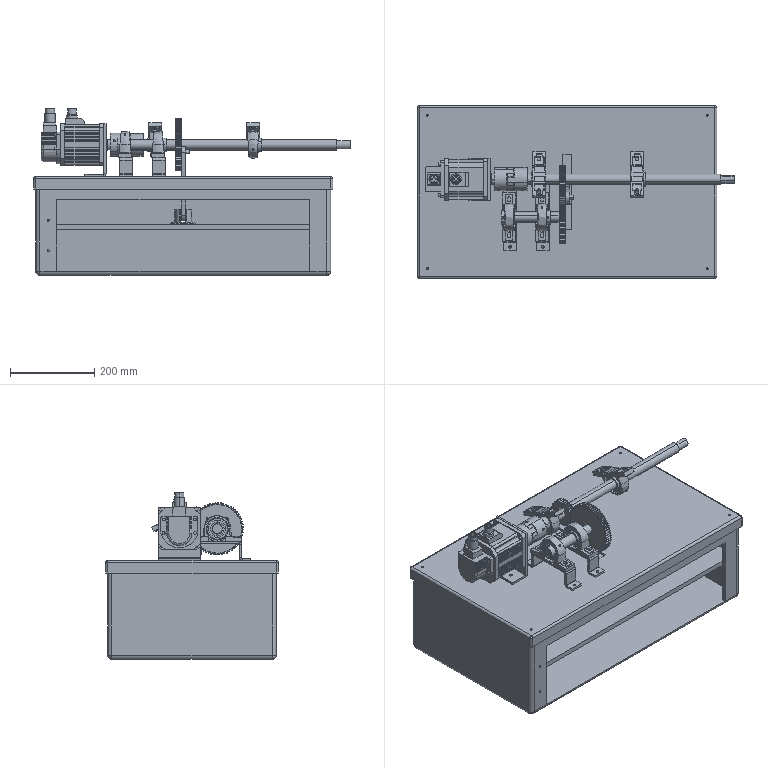Part | SolidWorks | features CompositeCurve 2 | 24 solids | 1807 faces | box 752 x 410 x 396 mm | volume 13592742 mm3 | cylinder 864 | plane 718 | cone 140 | sphere 40 | torus 33 | spline 12 | commonest cylinder face diameters 48 x124 24 x76 114.998 x61 124 x60 5 x44 10 x44